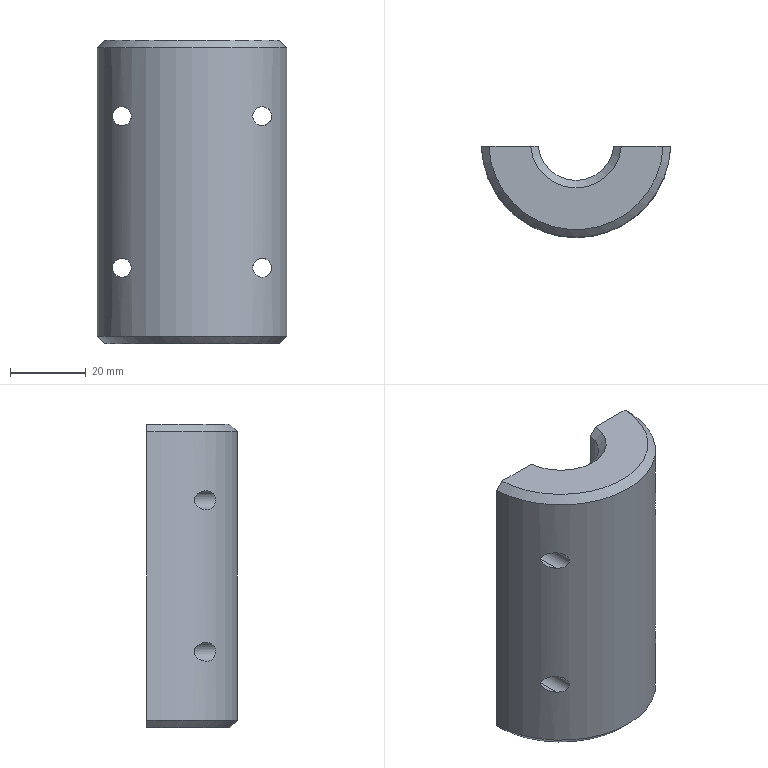Part | SolidWorks | features Chamfer 1, Extrusion 1, HoleWzd 1 | 1 solid | 18 faces | box 49.96 x 24 x 80 mm | volume 61914 mm3 | cylinder 10 | plane 4 | cone 4 | commonest cylinder face diameters 5 x8 20 x1 50 x1
STEP:
#1=CARTESIAN_POINT('',(-18.5,-16.815,17.5));
#2=VERTEX_POINT('',#1);
#3=CARTESIAN_POINT('',(-18.5,-16.815,22.5));
#4=VERTEX_POINT('',#3);
#5=CARTESIAN_POINT('',(-18.5,-16.815,17.5));
#6=CARTESIAN_POINT('',(-18.791,-16.495,17.5));
#7=CARTESIAN_POINT('',(-19.077,-16.163,17.551));
#8=CARTESIAN_POINT('',(-19.612,-15.509,17.743));
#9=CARTESIAN_POINT('',(-19.865,-15.183,17.884));
#10=CARTESIAN_POINT('',(-20.215,-14.711,18.174));
#11=CARTESIAN_POINT('',(-20.325,-14.558,18.284));
#12=CARTESIAN_POINT('',(-20.531,-14.266,18.533));
#13=CARTESIAN_POINT('',(-20.627,-14.126,18.675));
#14=CARTESIAN_POINT('',(-20.794,-13.878,18.991));
#15=CARTESIAN_POINT('',(-20.867,-13.768,19.171));
#16=CARTESIAN_POINT('',(-20.97,-13.611,19.564));
#17=CARTESIAN_POINT('',(-21.,-13.565,19.783));
#18=CARTESIAN_POINT('',(-21.,-13.565,20.109));
#19=CARTESIAN_POINT('',(-20.993,-13.576,20.22));
#20=CARTESIAN_POINT('',(-20.965,-13.619,20.432));
#21=CARTESIAN_POINT('',(-20.944,-13.651,20.535));
#22=CARTESIAN_POINT('',(-20.866,-13.771,20.834));
#23=CARTESIAN_POINT('',(-20.795,-13.878,21.009));
#24=CARTESIAN_POINT('',(-20.625,-14.129,21.329));
#25=CARTESIAN_POINT('',(-20.53,-14.267,21.467));
#26=CARTESIAN_POINT('',(-20.325,-14.557,21.716));
#27=CARTESIAN_POINT('',(-20.214,-14.712,21.826));
#28=CARTESIAN_POINT('',(-19.866,-15.182,22.116));
#29=CARTESIAN_POINT('',(-19.615,-15.505,22.256));
#30=CARTESIAN_POINT('',(-19.213,-15.997,22.4));
#31=CARTESIAN_POINT('',(-19.074,-16.163,22.437));
#32=CARTESIAN_POINT('',(-18.791,-16.491,22.487));
#33=CARTESIAN_POINT('',(-18.647,-16.653,22.5));
#34=CARTESIAN_POINT('',(-18.5,-16.815,22.5));
#35=B_SPLINE_CURVE_WITH_KNOTS('',3,(#5,#6,#7,#8,#9,#10,#11,#12,#13,#14,#15,#16,#17,#18,#19,#20,#21,#22,#23,#24,#25,#26,#27,#28,#29,#30,#31,#32,#33,#34),.UNSPECIFIED.,.F.,.F.,(4,2,2,2,2,2,2,2,2,2,2,2,2,2,4),(0.009381,0.01068,0.01197,0.01262,0.01327,0.01391,0.01456,0.01489,0.01521,0.01586,0.0165,0.01715,0.01845,0.0191,0.01974),.UNSPECIFIED.);
#36=EDGE_CURVE('',#2,#4,#35,.T.);
#37=ORIENTED_EDGE('',*,*,#36,.F.);
#38=CARTESIAN_POINT('',(-18.5,-1.,17.5));
#39=VERTEX_POINT('',#38);
#40=CARTESIAN_POINT('',(-18.5,-1.,17.5));
#41=DIRECTION('',(0.,1.,0.));
#42=VECTOR('',#41,1000.);
#43=LINE('',#40,#42);
#44=EDGE_CURVE('',#2,#39,#43,.T.);
#45=ORIENTED_EDGE('',*,*,#44,.T.);
#46=CARTESIAN_POINT('',(-18.5,-1.,22.5));
#47=VERTEX_POINT('',#46);
#48=CARTESIAN_POINT('',(-18.5,-1.,20.));
#49=DIRECTION('',(0.,1.,0.));
#50=DIRECTION('',(0.,0.,1.));
#51=AXIS2_PLACEMENT_3D('',#48,#49,#50);
#52=CIRCLE('',#51,2.5);
#53=EDGE_CURVE('',#39,#47,#52,.T.);
#54=ORIENTED_EDGE('',*,*,#53,.T.);
#55=CARTESIAN_POINT('',(-18.5,-1.,22.5));
#56=DIRECTION('',(0.,1.,0.));
#57=VECTOR('',#56,1000.);
#58=LINE('',#55,#57);
#59=EDGE_CURVE('',#4,#47,#58,.T.);
#60=ORIENTED_EDGE('',*,*,#59,.F.);
#61=EDGE_LOOP('',(#37,#45,#54,#60));
#62=FACE_OUTER_BOUND('',#61,.T.);
#63=CARTESIAN_POINT('',(-18.5,-1.,20.));
#64=DIRECTION('',(0.,1.,0.));
#65=DIRECTION('',(0.,0.,1.));
#66=AXIS2_PLACEMENT_3D('',#63,#64,#65);
#67=CYLINDRICAL_SURFACE('',#66,2.5);
#68=ADVANCED_FACE('',(#62),#67,.F.);
#69=CARTESIAN_POINT('',(18.5,-16.815,17.5));
#70=VERTEX_POINT('',#69);
#71=CARTESIAN_POINT('',(18.5,-16.815,22.5));
#72=VERTEX_POINT('',#71);
#73=CARTESIAN_POINT('',(18.5,-16.815,17.5));
#74=CARTESIAN_POINT('',(18.235,-17.107,17.5));
#75=CARTESIAN_POINT('',(17.966,-17.388,17.541));
#76=CARTESIAN_POINT('',(17.56,-17.796,17.679));
#77=CARTESIAN_POINT('',(17.424,-17.929,17.738));
#78=CARTESIAN_POINT('',(17.16,-18.181,17.884));
#79=CARTESIAN_POINT('',(17.031,-18.302,17.97));
#80=CARTESIAN_POINT('',(16.783,-18.53,18.176));
#81=CARTESIAN_POINT('',(16.663,-18.637,18.295));
#82=CARTESIAN_POINT('',(16.447,-18.828,18.563));
#83=CARTESIAN_POINT('',(16.348,-18.914,18.714));
#84=CARTESIAN_POINT('',(16.183,-19.056,19.044));
#85=CARTESIAN_POINT('',(16.116,-19.112,19.222));
#86=CARTESIAN_POINT('',(16.024,-19.189,19.602));
#87=CARTESIAN_POINT('',(16.,-19.209,19.796));
#88=CARTESIAN_POINT('',(16.,-19.21,20.193));
#89=CARTESIAN_POINT('',(16.023,-19.19,20.39));
#90=CARTESIAN_POINT('',(16.113,-19.115,20.768));
#91=CARTESIAN_POINT('',(16.18,-19.058,20.949));
#92=CARTESIAN_POINT('',(16.345,-18.917,21.28));
#93=CARTESIAN_POINT('',(16.444,-18.831,21.432));
#94=CARTESIAN_POINT('',(16.66,-18.64,21.702));
#95=CARTESIAN_POINT('',(16.78,-18.533,21.821));
#96=CARTESIAN_POINT('',(17.028,-18.305,22.027));
#97=CARTESIAN_POINT('',(17.157,-18.184,22.114));
#98=CARTESIAN_POINT('',(17.421,-17.932,22.26));
#99=CARTESIAN_POINT('',(17.557,-17.799,22.32));
#100=CARTESIAN_POINT('',(17.964,-17.391,22.458));
#101=CARTESIAN_POINT('',(18.233,-17.109,22.5));
#102=CARTESIAN_POINT('',(18.5,-16.815,22.5));
#103=B_SPLINE_CURVE_WITH_KNOTS('',3,(#73,#74,#75,#76,#77,#78,#79,#80,#81,#82,#83,#84,#85,#86,#87,#88,#89,#90,#91,#92,#93,#94,#95,#96,#97,#98,#99,#100,#101,#102),.UNSPECIFIED.,.F.,.F.,(4,2,2,2,2,2,2,2,2,2,2,2,2,2,4),(0.01037,0.01154,0.01213,0.01271,0.0133,0.01389,0.01447,0.01506,0.01565,0.01623,0.01682,0.01741,0.01799,0.01858,0.01975),.UNSPECIFIED.);
#104=EDGE_CURVE('',#70,#72,#103,.T.);
#105=ORIENTED_EDGE('',*,*,#104,.F.);
#106=CARTESIAN_POINT('',(18.5,-1.,17.5));
#107=VERTEX_POINT('',#106);
#108=CARTESIAN_POINT('',(18.5,-1.,17.5));
#109=DIRECTION('',(0.,1.,0.));
#110=VECTOR('',#109,1000.);
#111=LINE('',#108,#110);
#112=EDGE_CURVE('',#70,#107,#111,.T.);
#113=ORIENTED_EDGE('',*,*,#112,.T.);
#114=CARTESIAN_POINT('',(18.5,-1.,22.5));
#115=VERTEX_POINT('',#114);
#116=CARTESIAN_POINT('',(18.5,-1.,20.));
#117=DIRECTION('',(0.,1.,0.));
#118=DIRECTION('',(0.,0.,1.));
#119=AXIS2_PLACEMENT_3D('',#116,#117,#118);
#120=CIRCLE('',#119,2.5);
#121=EDGE_CURVE('',#107,#115,#120,.T.);
#122=ORIENTED_EDGE('',*,*,#121,.T.);
#123=CARTESIAN_POINT('',(18.5,-1.,22.5));
#124=DIRECTION('',(0.,1.,0.));
#125=VECTOR('',#124,1000.);
#126=LINE('',#123,#125);
#127=EDGE_CURVE('',#72,#115,#126,.T.);
#128=ORIENTED_EDGE('',*,*,#127,.F.);
#129=EDGE_LOOP('',(#105,#113,#122,#128));
#130=FACE_OUTER_BOUND('',#129,.T.);
#131=CARTESIAN_POINT('',(18.5,-1.,20.));
#132=DIRECTION('',(0.,1.,0.));
#133=DIRECTION('',(0.,0.,1.));
#134=AXIS2_PLACEMENT_3D('',#131,#132,#133);
#135=CYLINDRICAL_SURFACE('',#134,2.5);
#136=ADVANCED_FACE('',(#130),#135,.F.);
#137=CARTESIAN_POINT('',(18.5,-16.815,57.5));
#138=VERTEX_POINT('',#137);
#139=CARTESIAN_POINT('',(18.5,-16.815,62.5));
#140=VERTEX_POINT('',#139);
#141=CARTESIAN_POINT('',(18.5,-16.815,57.5));
#142=CARTESIAN_POINT('',(18.235,-17.107,57.5));
#143=CARTESIAN_POINT('',(17.966,-17.388,57.541));
#144=CARTESIAN_POINT('',(17.56,-17.796,57.679));
#145=CARTESIAN_POINT('',(17.424,-17.929,57.738));
#146=CARTESIAN_POINT('',(17.16,-18.181,57.884));
#147=CARTESIAN_POINT('',(17.031,-18.302,57.97));
#148=CARTESIAN_POINT('',(16.783,-18.53,58.176));
#149=CARTESIAN_POINT('',(16.663,-18.637,58.295));
#150=CARTESIAN_POINT('',(16.447,-18.828,58.563));
#151=CARTESIAN_POINT('',(16.348,-18.914,58.714));
#152=CARTESIAN_POINT('',(16.183,-19.056,59.044));
#153=CARTESIAN_POINT('',(16.116,-19.112,59.222));
#154=CARTESIAN_POINT('',(16.024,-19.189,59.602));
#155=CARTESIAN_POINT('',(16.,-19.209,59.796));
#156=CARTESIAN_POINT('',(16.,-19.21,60.193));
#157=CARTESIAN_POINT('',(16.023,-19.19,60.39));
#158=CARTESIAN_POINT('',(16.113,-19.115,60.768));
#159=CARTESIAN_POINT('',(16.18,-19.058,60.949));
#160=CARTESIAN_POINT('',(16.345,-18.917,61.28));
#161=CARTESIAN_POINT('',(16.444,-18.831,61.432));
#162=CARTESIAN_POINT('',(16.66,-18.64,61.702));
#163=CARTESIAN_POINT('',(16.78,-18.533,61.821));
#164=CARTESIAN_POINT('',(17.028,-18.305,62.027));
#165=CARTESIAN_POINT('',(17.157,-18.184,62.114));
#166=CARTESIAN_POINT('',(17.421,-17.932,62.26));
#167=CARTESIAN_POINT('',(17.557,-17.799,62.32));
#168=CARTESIAN_POINT('',(17.964,-17.391,62.458));
#169=CARTESIAN_POINT('',(18.233,-17.109,62.5));
#170=CARTESIAN_POINT('',(18.5,-16.815,62.5));
#171=B_SPLINE_CURVE_WITH_KNOTS('',3,(#141,#142,#143,#144,#145,#146,#147,#148,#149,#150,#151,#152,#153,#154,#155,#156,#157,#158,#159,#160,#161,#162,#163,#164,#165,#166,#167,#168,#169,#170),.UNSPECIFIED.,.F.,.F.,(4,2,2,2,2,2,2,2,2,2,2,2,2,2,4),(0.01037,0.01154,0.01213,0.01271,0.0133,0.01389,0.01447,0.01506,0.01565,0.01623,0.01682,0.01741,0.01799,0.01858,0.01975),.UNSPECIFIED.);
#172=EDGE_CURVE('',#138,#140,#171,.T.);
#173=ORIENTED_EDGE('',*,*,#172,.F.);
#174=CARTESIAN_POINT('',(18.5,-1.,57.5));
#175=VERTEX_POINT('',#174);
#176=CARTESIAN_POINT('',(18.5,-1.,57.5));
#177=DIRECTION('',(0.,1.,0.));
#178=VECTOR('',#177,1000.);
#179=LINE('',#176,#178);
#180=EDGE_CURVE('',#138,#175,#179,.T.);
#181=ORIENTED_EDGE('',*,*,#180,.T.);
#182=CARTESIAN_POINT('',(18.5,-1.,62.5));
#183=VERTEX_POINT('',#182);
#184=CARTESIAN_POINT('',(18.5,-1.,60.));
#185=DIRECTION('',(0.,1.,0.));
#186=DIRECTION('',(0.,0.,1.));
#187=AXIS2_PLACEMENT_3D('',#184,#185,#186);
#188=CIRCLE('',#187,2.5);
#189=EDGE_CURVE('',#175,#183,#188,.T.);
#190=ORIENTED_EDGE('',*,*,#189,.T.);
#191=CARTESIAN_POINT('',(18.5,-1.,62.5));
#192=DIRECTION('',(0.,1.,0.));
#193=VECTOR('',#192,1000.);
#194=LINE('',#191,#193);
#195=EDGE_CURVE('',#140,#183,#194,.T.);
#196=ORIENTED_EDGE('',*,*,#195,.F.);
#197=EDGE_LOOP('',(#173,#181,#190,#196));
#198=FACE_OUTER_BOUND('',#197,.T.);
#199=CARTESIAN_POINT('',(18.5,-1.,60.));
#200=DIRECTION('',(0.,1.,0.));
#201=DIRECTION('',(0.,0.,1.));
#202=AXIS2_PLACEMENT_3D('',#199,#200,#201);
#203=CYLINDRICAL_SURFACE('',#202,2.5);
#204=ADVANCED_FACE('',(#198),#203,.F.);
#205=CARTESIAN_POINT('',(-18.5,-16.815,57.5));
#206=VERTEX_POINT('',#205);
#207=CARTESIAN_POINT('',(-18.5,-16.815,62.5));
#208=VERTEX_POINT('',#207);
#209=CARTESIAN_POINT('',(-18.5,-16.815,57.5));
#210=CARTESIAN_POINT('',(-18.791,-16.495,57.5));
#211=CARTESIAN_POINT('',(-19.077,-16.163,57.551));
#212=CARTESIAN_POINT('',(-19.612,-15.509,57.743));
#213=CARTESIAN_POINT('',(-19.865,-15.183,57.884));
#214=CARTESIAN_POINT('',(-20.215,-14.711,58.174));
#215=CARTESIAN_POINT('',(-20.325,-14.558,58.284));
#216=CARTESIAN_POINT('',(-20.531,-14.266,58.533));
#217=CARTESIAN_POINT('',(-20.627,-14.126,58.675));
#218=CARTESIAN_POINT('',(-20.794,-13.878,58.991));
#219=CARTESIAN_POINT('',(-20.867,-13.768,59.171));
#220=CARTESIAN_POINT('',(-20.97,-13.611,59.564));
#221=CARTESIAN_POINT('',(-21.,-13.565,59.783));
#222=CARTESIAN_POINT('',(-21.,-13.565,60.109));
#223=CARTESIAN_POINT('',(-20.993,-13.576,60.22));
#224=CARTESIAN_POINT('',(-20.965,-13.619,60.432));
#225=CARTESIAN_POINT('',(-20.944,-13.651,60.535));
#226=CARTESIAN_POINT('',(-20.866,-13.771,60.834));
#227=CARTESIAN_POINT('',(-20.795,-13.878,61.009));
#228=CARTESIAN_POINT('',(-20.625,-14.129,61.329));
#229=CARTESIAN_POINT('',(-20.53,-14.267,61.467));
#230=CARTESIAN_POINT('',(-20.325,-14.557,61.716));
#231=CARTESIAN_POINT('',(-20.214,-14.712,61.826));
#232=CARTESIAN_POINT('',(-19.866,-15.182,62.116));
#233=CARTESIAN_POINT('',(-19.615,-15.505,62.256));
#234=CARTESIAN_POINT('',(-19.213,-15.997,62.4));
#235=CARTESIAN_POINT('',(-19.074,-16.163,62.437));
#236=CARTESIAN_POINT('',(-18.791,-16.491,62.487));
#237=CARTESIAN_POINT('',(-18.647,-16.653,62.5));
#238=CARTESIAN_POINT('',(-18.5,-16.815,62.5));
#239=B_SPLINE_CURVE_WITH_KNOTS('',3,(#209,#210,#211,#212,#213,#214,#215,#216,#217,#218,#219,#220,#221,#222,#223,#224,#225,#226,#227,#228,#229,#230,#231,#232,#233,#234,#235,#236,#237,#238),.UNSPECIFIED.,.F.,.F.,(4,2,2,2,2,2,2,2,2,2,2,2,2,2,4),(0.009381,0.01068,0.01197,0.01262,0.01327,0.01391,0.01456,0.01489,0.01521,0.01586,0.0165,0.01715,0.01845,0.0191,0.01974),.UNSPECIFIED.);
#240=EDGE_CURVE('',#206,#208,#239,.T.);
#241=ORIENTED_EDGE('',*,*,#240,.F.);
#242=CARTESIAN_POINT('',(-18.5,-1.,57.5));
#243=VERTEX_POINT('',#242);
#244=CARTESIAN_POINT('',(-18.5,-1.,57.5));
#245=DIRECTION('',(0.,1.,0.));
#246=VECTOR('',#245,1000.);
#247=LINE('',#244,#246);
#248=EDGE_CURVE('',#206,#243,#247,.T.);
#249=ORIENTED_EDGE('',*,*,#248,.T.);
#250=CARTESIAN_POINT('',(-18.5,-1.,62.5));
#251=VERTEX_POINT('',#250);
#252=CARTESIAN_POINT('',(-18.5,-1.,60.));
#253=DIRECTION('',(0.,1.,0.));
#254=DIRECTION('',(0.,0.,1.));
#255=AXIS2_PLACEMENT_3D('',#252,#253,#254);
#256=CIRCLE('',#255,2.5);
#257=EDGE_CURVE('',#243,#251,#256,.T.);
#258=ORIENTED_EDGE('',*,*,#257,.T.);
#259=CARTESIAN_POINT('',(-18.5,-1.,62.5));
#260=DIRECTION('',(0.,1.,0.));
#261=VECTOR('',#260,1000.);
#262=LINE('',#259,#261);
#263=EDGE_CURVE('',#208,#251,#262,.T.);
#264=ORIENTED_EDGE('',*,*,#263,.F.);
#265=EDGE_LOOP('',(#241,#249,#258,#264));
#266=FACE_OUTER_BOUND('',#265,.T.);
#267=CARTESIAN_POINT('',(-18.5,-1.,60.));
#268=DIRECTION('',(0.,1.,0.));
#269=DIRECTION('',(0.,0.,1.));
#270=AXIS2_PLACEMENT_3D('',#267,#268,#269);
#271=CYLINDRICAL_SURFACE('',#270,2.5);
#272=ADVANCED_FACE('',(#266),#271,.F.);
#273=CARTESIAN_POINT('',(-9.95,-1.,78.));
#274=VERTEX_POINT('',#273);
#275=CARTESIAN_POINT('',(-9.95,-1.,2.));
#276=VERTEX_POINT('',#275);
#277=CARTESIAN_POINT('',(-9.95,-1.,80.));
#278=DIRECTION('',(0.,0.,-1.));
#279=VECTOR('',#278,1000.);
#280=LINE('',#277,#279);
#281=EDGE_CURVE('',#274,#276,#280,.T.);
#282=ORIENTED_EDGE('',*,*,#281,.F.);
#283=CARTESIAN_POINT('',(9.95,-1.,78.));
#284=VERTEX_POINT('',#283);
#285=CARTESIAN_POINT('',(0.,0.,78.));
#286=DIRECTION('',(0.,0.,1.));
#287=DIRECTION('',(1.,0.,0.));
#288=AXIS2_PLACEMENT_3D('',#285,#286,#287);
#289=CIRCLE('',#288,10.);
#290=EDGE_CURVE('',#274,#284,#289,.T.);
#291=ORIENTED_EDGE('',*,*,#290,.T.);
#292=CARTESIAN_POINT('',(9.95,-1.,2.));
#293=VERTEX_POINT('',#292);
#294=CARTESIAN_POINT('',(9.95,-1.,80.));
#295=DIRECTION('',(0.,0.,-1.));
#296=VECTOR('',#295,1000.);
#297=LINE('',#294,#296);
#298=EDGE_CURVE('',#284,#293,#297,.T.);
#299=ORIENTED_EDGE('',*,*,#298,.T.);
#300=CARTESIAN_POINT('',(0.,0.,2.));
#301=DIRECTION('',(0.,0.,-1.));
#302=DIRECTION('',(1.,0.,0.));
#303=AXIS2_PLACEMENT_3D('',#300,#301,#302);
#304=CIRCLE('',#303,10.);
#305=EDGE_CURVE('',#293,#276,#304,.T.);
#306=ORIENTED_EDGE('',*,*,#305,.T.);
#307=EDGE_LOOP('',(#282,#291,#299,#306));
#308=FACE_OUTER_BOUND('',#307,.T.);
#309=CARTESIAN_POINT('',(0.,0.,80.));
#310=DIRECTION('',(0.,0.,-1.));
#311=DIRECTION('',(-1.,0.,0.));
#312=AXIS2_PLACEMENT_3D('',#309,#310,#311);
#313=CYLINDRICAL_SURFACE('',#312,10.);
#314=ADVANCED_FACE('',(#308),#313,.F.);
#315=CARTESIAN_POINT('',(-18.5,-1.,20.));
#316=DIRECTION('',(0.,1.,0.));
#317=DIRECTION('',(0.,0.,1.));
#318=AXIS2_PLACEMENT_3D('',#315,#316,#317);
#319=CIRCLE('',#318,2.5);
#320=EDGE_CURVE('',#47,#39,#319,.T.);
#321=ORIENTED_EDGE('',*,*,#320,.F.);
#322=ORIENTED_EDGE('',*,*,#53,.F.);
#323=EDGE_LOOP('',(#321,#322));
#324=FACE_BOUND('',#323,.T.);
#325=CARTESIAN_POINT('',(-18.5,-1.,60.));
#326=DIRECTION('',(0.,1.,0.));
#327=DIRECTION('',(0.,0.,1.));
#328=AXIS2_PLACEMENT_3D('',#325,#326,#327);
#329=CIRCLE('',#328,2.5);
#330=EDGE_CURVE('',#251,#243,#329,.T.);
#331=ORIENTED_EDGE('',*,*,#330,.F.);
#332=ORIENTED_EDGE('',*,*,#257,.F.);
#333=EDGE_LOOP('',(#331,#332));
#334=FACE_BOUND('',#333,.T.);
#335=CARTESIAN_POINT('',(-24.98,-1.,78.));
#336=VERTEX_POINT('',#335);
#337=CARTESIAN_POINT('',(-24.98,-1.,2.));
#338=VERTEX_POINT('',#337);
#339=CARTESIAN_POINT('',(-24.98,-1.,80.));
#340=DIRECTION('',(0.,0.,-1.));
#341=VECTOR('',#340,1000.);
#342=LINE('',#339,#341);
#343=EDGE_CURVE('',#336,#338,#342,.T.);
#344=ORIENTED_EDGE('',*,*,#343,.F.);
#345=CARTESIAN_POINT('',(-22.978,-1.,80.));
#346=VERTEX_POINT('',#345);
#347=CARTESIAN_POINT('',(-24.98,-1.,78.));
#348=CARTESIAN_POINT('',(-24.313,-1.,78.667));
#349=CARTESIAN_POINT('',(-23.646,-1.,79.333));
#350=CARTESIAN_POINT('',(-22.978,-1.,80.));
#351=B_SPLINE_CURVE_WITH_KNOTS('',3,(#347,#348,#349,#350),.UNSPECIFIED.,.F.,.F.,(4,4),(0.,0.00283),.UNSPECIFIED.);
#352=EDGE_CURVE('',#336,#346,#351,.T.);
#353=ORIENTED_EDGE('',*,*,#352,.T.);
#354=CARTESIAN_POINT('',(-11.958,-1.,80.));
#355=VERTEX_POINT('',#354);
#356=CARTESIAN_POINT('',(-24.98,-1.,80.));
#357=DIRECTION('',(-1.,0.,0.));
#358=VECTOR('',#357,1000.);
#359=LINE('',#356,#358);
#360=EDGE_CURVE('',#355,#346,#359,.T.);
#361=ORIENTED_EDGE('',*,*,#360,.F.);
#362=CARTESIAN_POINT('',(-11.958,-1.,80.));
#363=CARTESIAN_POINT('',(-11.289,-1.,79.333));
#364=CARTESIAN_POINT('',(-10.62,-1.,78.666));
#365=CARTESIAN_POINT('',(-9.95,-1.,78.));
#366=B_SPLINE_CURVE_WITH_KNOTS('',3,(#362,#363,#364,#365),.UNSPECIFIED.,.F.,.F.,(4,4),(0.,0.002834),.UNSPECIFIED.);
#367=EDGE_CURVE('',#355,#274,#366,.T.);
#368=ORIENTED_EDGE('',*,*,#367,.T.);
#369=ORIENTED_EDGE('',*,*,#281,.T.);
#370=CARTESIAN_POINT('',(-11.958,-1.,0.));
#371=VERTEX_POINT('',#370);
#372=CARTESIAN_POINT('',(-9.95,-1.,2.));
#373=CARTESIAN_POINT('',(-10.62,-1.,1.334));
#374=CARTESIAN_POINT('',(-11.289,-1.,0.6669));
#375=CARTESIAN_POINT('',(-11.958,-1.,0.));
#376=B_SPLINE_CURVE_WITH_KNOTS('',3,(#372,#373,#374,#375),.UNSPECIFIED.,.F.,.F.,(4,4),(0.,0.002834),.UNSPECIFIED.);
#377=EDGE_CURVE('',#276,#371,#376,.T.);
#378=ORIENTED_EDGE('',*,*,#377,.T.);
#379=CARTESIAN_POINT('',(-22.978,-1.,0.));
#380=VERTEX_POINT('',#379);
#381=CARTESIAN_POINT('',(-24.98,-1.,0.));
#382=DIRECTION('',(-1.,0.,0.));
#383=VECTOR('',#382,1000.);
#384=LINE('',#381,#383);
#385=EDGE_CURVE('',#371,#380,#384,.T.);
#386=ORIENTED_EDGE('',*,*,#385,.T.);
#387=CARTESIAN_POINT('',(-22.978,-1.,0.));
#388=CARTESIAN_POINT('',(-23.646,-1.,0.6666));
#389=CARTESIAN_POINT('',(-24.313,-1.,1.333));
#390=CARTESIAN_POINT('',(-24.98,-1.,2.));
#391=B_SPLINE_CURVE_WITH_KNOTS('',3,(#387,#388,#389,#390),.UNSPECIFIED.,.F.,.F.,(4,4),(0.,0.00283),.UNSPECIFIED.);
#392=EDGE_CURVE('',#380,#338,#391,.T.);
#393=ORIENTED_EDGE('',*,*,#392,.T.);
#394=EDGE_LOOP('',(#344,#353,#361,#368,#369,#378,#386,#393));
#395=FACE_OUTER_BOUND('',#394,.T.);
#396=CARTESIAN_POINT('',(-24.98,-1.,80.));
#397=DIRECTION('',(0.,-1.,0.));
#398=DIRECTION('',(0.,0.,-1.));
#399=AXIS2_PLACEMENT_3D('',#396,#397,#398);
#400=PLANE('',#399);
#401=ADVANCED_FACE('',(#324,#334,#395),#400,.F.);
#402=CARTESIAN_POINT('',(-18.5,-16.815,22.5));
#403=CARTESIAN_POINT('',(-18.233,-17.108,22.5));
#404=CARTESIAN_POINT('',(-17.965,-17.39,22.459));
#405=CARTESIAN_POINT('',(-17.561,-17.795,22.321));
#406=CARTESIAN_POINT('',(-17.425,-17.928,22.262));
#407=CARTESIAN_POINT('',(-17.16,-18.182,22.116));
#408=CARTESIAN_POINT('',(-17.031,-18.303,22.029));
#409=CARTESIAN_POINT('',(-16.783,-18.53,21.824));
#410=CARTESIAN_POINT('',(-16.663,-18.638,21.704));
#411=CARTESIAN_POINT('',(-16.446,-18.829,21.436));
#412=CARTESIAN_POINT('',(-16.348,-18.914,21.287));
#413=CARTESIAN_POINT('',(-16.181,-19.057,20.953));
#414=CARTESIAN_POINT('',(-16.116,-19.113,20.776));
#415=CARTESIAN_POINT('',(-16.024,-19.189,20.397));
#416=CARTESIAN_POINT('',(-16.,-19.209,20.2));
#417=CARTESIAN_POINT('',(-16.,-19.21,19.805));
#418=CARTESIAN_POINT('',(-16.024,-19.19,19.606));
#419=CARTESIAN_POINT('',(-16.114,-19.114,19.229));
#420=CARTESIAN_POINT('',(-16.181,-19.057,19.047));
#421=CARTESIAN_POINT('',(-16.347,-18.916,18.717));
#422=CARTESIAN_POINT('',(-16.446,-18.829,18.564));
#423=CARTESIAN_POINT('',(-16.663,-18.638,18.296));
#424=CARTESIAN_POINT('',(-16.78,-18.532,18.178));
#425=CARTESIAN_POINT('',(-17.03,-18.304,17.972));
#426=CARTESIAN_POINT('',(-17.16,-18.182,17.884));
#427=CARTESIAN_POINT('',(-17.423,-17.929,17.739));
#428=CARTESIAN_POINT('',(-17.557,-17.798,17.68));
#429=CARTESIAN_POINT('',(-17.829,-17.526,17.588));
#430=CARTESIAN_POINT('',(-17.966,-17.386,17.554));
#431=CARTESIAN_POINT('',(-18.235,-17.103,17.51));
#432=CARTESIAN_POINT('',(-18.368,-16.96,17.5));
#433=CARTESIAN_POINT('',(-18.5,-16.815,17.5));
#434=B_SPLINE_CURVE_WITH_KNOTS('',3,(#402,#403,#404,#405,#406,#407,#408,#409,#410,#411,#412,#413,#414,#415,#416,#417,#418,#419,#420,#421,#422,#423,#424,#425,#426,#427,#428,#429,#430,#431,#432,#433),.UNSPECIFIED.,.F.,.F.,(4,2,2,2,2,2,2,2,2,2,2,2,2,2,2,4),(0.,0.001173,0.001759,0.002345,0.002931,0.003518,0.004104,0.00469,0.005277,0.005863,0.006449,0.007035,0.007622,0.008208,0.008794,0.009381),.UNSPECIFIED.);
#435=EDGE_CURVE('',#4,#2,#434,.T.);
#436=ORIENTED_EDGE('',*,*,#435,.T.);
#437=ORIENTED_EDGE('',*,*,#36,.T.);
#438=EDGE_LOOP('',(#436,#437));
#439=FACE_BOUND('',#438,.T.);
#440=CARTESIAN_POINT('',(18.5,-16.815,22.5));
#441=CARTESIAN_POINT('',(18.795,-16.491,22.5));
#442=CARTESIAN_POINT('',(19.075,-16.165,22.449));
#443=CARTESIAN_POINT('',(19.61,-15.512,22.258));
#444=CARTESIAN_POINT('',(19.866,-15.182,22.115));
#445=CARTESIAN_POINT('',(20.213,-14.713,21.827));
#446=CARTESIAN_POINT('',(20.323,-14.56,21.718));
#447=CARTESIAN_POINT('',(20.531,-14.266,21.467));
#448=CARTESIAN_POINT('',(20.626,-14.128,21.327));
#449=CARTESIAN_POINT('',(20.794,-13.879,21.01));
#450=CARTESIAN_POINT('',(20.867,-13.769,20.831));
#451=CARTESIAN_POINT('',(20.97,-13.611,20.436));
#452=CARTESIAN_POINT('',(21.,-13.564,20.219));
#453=CARTESIAN_POINT('',(21.,-13.565,19.888));
#454=CARTESIAN_POINT('',(20.993,-13.576,19.78));
#455=CARTESIAN_POINT('',(20.965,-13.619,19.567));
#456=CARTESIAN_POINT('',(20.944,-13.651,19.463));
#457=CARTESIAN_POINT('',(20.866,-13.77,19.168));
#458=CARTESIAN_POINT('',(20.793,-13.88,18.989));
#459=CARTESIAN_POINT('',(20.626,-14.128,18.672));
#460=CARTESIAN_POINT('',(20.531,-14.266,18.533));
#461=CARTESIAN_POINT('',(20.324,-14.56,18.282));
#462=CARTESIAN_POINT('',(20.214,-14.712,18.174));
#463=CARTESIAN_POINT('',(19.868,-15.18,17.886));
#464=CARTESIAN_POINT('',(19.612,-15.509,17.743));
#465=CARTESIAN_POINT('',(19.21,-16.,17.599));
#466=CARTESIAN_POINT('',(19.073,-16.164,17.562));
#467=CARTESIAN_POINT('',(18.791,-16.49,17.513));
#468=CARTESIAN_POINT('',(18.646,-16.654,17.5));
#469=CARTESIAN_POINT('',(18.5,-16.815,17.5));
#470=B_SPLINE_CURVE_WITH_KNOTS('',3,(#440,#441,#442,#443,#444,#445,#446,#447,#448,#449,#450,#451,#452,#453,#454,#455,#456,#457,#458,#459,#460,#461,#462,#463,#464,#465,#466,#467,#468,#469),.UNSPECIFIED.,.F.,.F.,(4,2,2,2,2,2,2,2,2,2,2,2,2,2,4),(0.,0.001296,0.002592,0.00324,0.003888,0.004535,0.005183,0.005507,0.005831,0.006479,0.007127,0.007775,0.009071,0.009719,0.01037),.UNSPECIFIED.);
#471=EDGE_CURVE('',#72,#70,#470,.T.);
#472=ORIENTED_EDGE('',*,*,#471,.T.);
#473=ORIENTED_EDGE('',*,*,#104,.T.);
#474=EDGE_LOOP('',(#472,#473));
#475=FACE_BOUND('',#474,.T.);
#476=CARTESIAN_POINT('',(18.5,-16.815,62.5));
#477=CARTESIAN_POINT('',(18.795,-16.491,62.5));
#478=CARTESIAN_POINT('',(19.075,-16.165,62.449));
#479=CARTESIAN_POINT('',(19.61,-15.512,62.258));
#480=CARTESIAN_POINT('',(19.866,-15.182,62.115));
#481=CARTESIAN_POINT('',(20.213,-14.713,61.827));
#482=CARTESIAN_POINT('',(20.323,-14.56,61.718));
#483=CARTESIAN_POINT('',(20.531,-14.266,61.467));
#484=CARTESIAN_POINT('',(20.626,-14.128,61.327));
#485=CARTESIAN_POINT('',(20.794,-13.879,61.01));
#486=CARTESIAN_POINT('',(20.867,-13.769,60.831));
#487=CARTESIAN_POINT('',(20.97,-13.611,60.436));
#488=CARTESIAN_POINT('',(21.,-13.564,60.219));
#489=CARTESIAN_POINT('',(21.,-13.565,59.888));
#490=CARTESIAN_POINT('',(20.993,-13.576,59.78));
#491=CARTESIAN_POINT('',(20.965,-13.619,59.567));
#492=CARTESIAN_POINT('',(20.944,-13.651,59.463));
#493=CARTESIAN_POINT('',(20.866,-13.77,59.168));
#494=CARTESIAN_POINT('',(20.793,-13.88,58.989));
#495=CARTESIAN_POINT('',(20.626,-14.128,58.672));
#496=CARTESIAN_POINT('',(20.531,-14.266,58.533));
#497=CARTESIAN_POINT('',(20.324,-14.56,58.282));
#498=CARTESIAN_POINT('',(20.214,-14.712,58.174));
#499=CARTESIAN_POINT('',(19.868,-15.18,57.886));
#500=CARTESIAN_POINT('',(19.612,-15.509,57.743));
#501=CARTESIAN_POINT('',(19.21,-16.,57.599));
#502=CARTESIAN_POINT('',(19.073,-16.164,57.562));
#503=CARTESIAN_POINT('',(18.791,-16.49,57.513));
#504=CARTESIAN_POINT('',(18.646,-16.654,57.5));
#505=CARTESIAN_POINT('',(18.5,-16.815,57.5));
#506=B_SPLINE_CURVE_WITH_KNOTS('',3,(#476,#477,#478,#479,#480,#481,#482,#483,#484,#485,#486,#487,#488,#489,#490,#491,#492,#493,#494,#495,#496,#497,#498,#499,#500,#501,#502,#503,#504,#505),.UNSPECIFIED.,.F.,.F.,(4,2,2,2,2,2,2,2,2,2,2,2,2,2,4),(0.,0.001296,0.002592,0.00324,0.003888,0.004535,0.005183,0.005507,0.005831,0.006479,0.007127,0.007775,0.009071,0.009719,0.01037),.UNSPECIFIED.);
#507=EDGE_CURVE('',#140,#138,#506,.T.);
#508=ORIENTED_EDGE('',*,*,#507,.T.);
#509=ORIENTED_EDGE('',*,*,#172,.T.);
#510=EDGE_LOOP('',(#508,#509));
#511=FACE_BOUND('',#510,.T.);
#512=CARTESIAN_POINT('',(-18.5,-16.815,62.5));
#513=CARTESIAN_POINT('',(-18.233,-17.108,62.5));
#514=CARTESIAN_POINT('',(-17.965,-17.39,62.459));
#515=CARTESIAN_POINT('',(-17.561,-17.795,62.321));
#516=CARTESIAN_POINT('',(-17.425,-17.928,62.262));
#517=CARTESIAN_POINT('',(-17.16,-18.182,62.116));
#518=CARTESIAN_POINT('',(-17.031,-18.303,62.029));
#519=CARTESIAN_POINT('',(-16.783,-18.53,61.824));
#520=CARTESIAN_POINT('',(-16.663,-18.638,61.704));
#521=CARTESIAN_POINT('',(-16.446,-18.829,61.436));
#522=CARTESIAN_POINT('',(-16.348,-18.914,61.287));
#523=CARTESIAN_POINT('',(-16.181,-19.057,60.953));
#524=CARTESIAN_POINT('',(-16.116,-19.113,60.776));
#525=CARTESIAN_POINT('',(-16.024,-19.189,60.397));
#526=CARTESIAN_POINT('',(-16.,-19.209,60.2));
#527=CARTESIAN_POINT('',(-16.,-19.21,59.805));
#528=CARTESIAN_POINT('',(-16.024,-19.19,59.606));
#529=CARTESIAN_POINT('',(-16.114,-19.114,59.229));
#530=CARTESIAN_POINT('',(-16.181,-19.057,59.047));
#531=CARTESIAN_POINT('',(-16.347,-18.916,58.717));
#532=CARTESIAN_POINT('',(-16.446,-18.829,58.564));
#533=CARTESIAN_POINT('',(-16.663,-18.638,58.296));
#534=CARTESIAN_POINT('',(-16.78,-18.532,58.178));
#535=CARTESIAN_POINT('',(-17.03,-18.304,57.972));
#536=CARTESIAN_POINT('',(-17.16,-18.182,57.884));
#537=CARTESIAN_POINT('',(-17.423,-17.929,57.739));
#538=CARTESIAN_POINT('',(-17.557,-17.798,57.68));
#539=CARTESIAN_POINT('',(-17.829,-17.526,57.588));
#540=CARTESIAN_POINT('',(-17.966,-17.386,57.554));
#541=CARTESIAN_POINT('',(-18.235,-17.103,57.51));
#542=CARTESIAN_POINT('',(-18.368,-16.96,57.5));
#543=CARTESIAN_POINT('',(-18.5,-16.815,57.5));
#544=B_SPLINE_CURVE_WITH_KNOTS('',3,(#512,#513,#514,#515,#516,#517,#518,#519,#520,#521,#522,#523,#524,#525,#526,#527,#528,#529,#530,#531,#532,#533,#534,#535,#536,#537,#538,#539,#540,#541,#542,#543),.UNSPECIFIED.,.F.,.F.,(4,2,2,2,2,2,2,2,2,2,2,2,2,2,2,4),(0.,0.001173,0.001759,0.002345,0.002931,0.003518,0.004104,0.00469,0.005277,0.005863,0.006449,0.007035,0.007622,0.008208,0.008794,0.009381),.UNSPECIFIED.);
#545=EDGE_CURVE('',#208,#206,#544,.T.);
#546=ORIENTED_EDGE('',*,*,#545,.T.);
#547=ORIENTED_EDGE('',*,*,#240,.T.);
#548=EDGE_LOOP('',(#546,#547));
#549=FACE_BOUND('',#548,.T.);
#550=CARTESIAN_POINT('',(24.98,-1.,78.));
#551=VERTEX_POINT('',#550);
#552=CARTESIAN_POINT('',(24.98,-1.,2.));
#553=VERTEX_POINT('',#552);
#554=CARTESIAN_POINT('',(24.98,-1.,80.));
#555=DIRECTION('',(0.,0.,-1.));
#556=VECTOR('',#555,1000.);
#557=LINE('',#554,#556);
#558=EDGE_CURVE('',#551,#553,#557,.T.);
#559=ORIENTED_EDGE('',*,*,#558,.F.);
#560=CARTESIAN_POINT('',(0.,0.,78.));
#561=DIRECTION('',(0.,0.,-1.));
#562=DIRECTION('',(1.,0.,0.));
#563=AXIS2_PLACEMENT_3D('',#560,#561,#562);
#564=CIRCLE('',#563,25.);
#565=EDGE_CURVE('',#551,#336,#564,.T.);
#566=ORIENTED_EDGE('',*,*,#565,.T.);
#567=ORIENTED_EDGE('',*,*,#343,.T.);
#568=CARTESIAN_POINT('',(0.,0.,2.));
#569=DIRECTION('',(0.,0.,1.));
#570=DIRECTION('',(1.,0.,0.));
#571=AXIS2_PLACEMENT_3D('',#568,#569,#570);
#572=CIRCLE('',#571,25.);
#573=EDGE_CURVE('',#338,#553,#572,.T.);
#574=ORIENTED_EDGE('',*,*,#573,.T.);
#575=EDGE_LOOP('',(#559,#566,#567,#574));
#576=FACE_OUTER_BOUND('',#575,.T.);
#577=CARTESIAN_POINT('',(0.,0.,80.));
#578=DIRECTION('',(0.,0.,-1.));
#579=DIRECTION('',(-1.,0.,0.));
#580=AXIS2_PLACEMENT_3D('',#577,#578,#579);
#581=CYLINDRICAL_SURFACE('',#580,25.);
#582=ADVANCED_FACE('',(#439,#475,#511,#549,#576),#581,.T.);
#583=CARTESIAN_POINT('',(18.5,-1.,20.));
#584=DIRECTION('',(0.,1.,0.));
#585=DIRECTION('',(0.,0.,1.));
#586=AXIS2_PLACEMENT_3D('',#583,#584,#585);
#587=CIRCLE('',#586,2.5);
#588=EDGE_CURVE('',#115,#107,#587,.T.);
#589=ORIENTED_EDGE('',*,*,#588,.F.);
#590=ORIENTED_EDGE('',*,*,#121,.F.);
#591=EDGE_LOOP('',(#589,#590));
#592=FACE_BOUND('',#591,.T.);
#593=CARTESIAN_POINT('',(18.5,-1.,60.));
#594=DIRECTION('',(0.,1.,0.));
#595=DIRECTION('',(0.,0.,1.));
#596=AXIS2_PLACEMENT_3D('',#593,#594,#595);
#597=CIRCLE('',#596,2.5);
#598=EDGE_CURVE('',#183,#175,#597,.T.);
#599=ORIENTED_EDGE('',*,*,#598,.F.);
#600=ORIENTED_EDGE('',*,*,#189,.F.);
#601=EDGE_LOOP('',(#599,#600));
#602=FACE_BOUND('',#601,.T.);
#603=CARTESIAN_POINT('',(22.978,-1.,80.));
#604=VERTEX_POINT('',#603);
#605=CARTESIAN_POINT('',(11.958,-1.,80.));
#606=VERTEX_POINT('',#605);
#607=CARTESIAN_POINT('',(9.95,-1.,80.));
#608=DIRECTION('',(-1.,0.,0.));
#609=VECTOR('',#608,1000.);
#610=LINE('',#607,#609);
#611=EDGE_CURVE('',#604,#606,#610,.T.);
#612=ORIENTED_EDGE('',*,*,#611,.F.);
#613=CARTESIAN_POINT('',(22.978,-1.,80.));
#614=CARTESIAN_POINT('',(23.646,-1.,79.333));
#615=CARTESIAN_POINT('',(24.313,-1.,78.667));
#616=CARTESIAN_POINT('',(24.98,-1.,78.));
#617=B_SPLINE_CURVE_WITH_KNOTS('',3,(#613,#614,#615,#616),.UNSPECIFIED.,.F.,.F.,(4,4),(0.,0.00283),.UNSPECIFIED.);
#618=EDGE_CURVE('',#604,#551,#617,.T.);
#619=ORIENTED_EDGE('',*,*,#618,.T.);
#620=ORIENTED_EDGE('',*,*,#558,.T.);
#621=CARTESIAN_POINT('',(22.978,-1.,0.));
#622=VERTEX_POINT('',#621);
#623=CARTESIAN_POINT('',(24.98,-1.,2.));
#624=CARTESIAN_POINT('',(24.313,-1.,1.333));
#625=CARTESIAN_POINT('',(23.646,-1.,0.6666));
#626=CARTESIAN_POINT('',(22.978,-1.,0.));
#627=B_SPLINE_CURVE_WITH_KNOTS('',3,(#623,#624,#625,#626),.UNSPECIFIED.,.F.,.F.,(4,4),(0.,0.00283),.UNSPECIFIED.);
#628=EDGE_CURVE('',#553,#622,#627,.T.);
#629=ORIENTED_EDGE('',*,*,#628,.T.);
#630=CARTESIAN_POINT('',(11.958,-1.,0.));
#631=VERTEX_POINT('',#630);
#632=CARTESIAN_POINT('',(9.95,-1.,0.));
#633=DIRECTION('',(-1.,0.,0.));
#634=VECTOR('',#633,1000.);
#635=LINE('',#632,#634);
#636=EDGE_CURVE('',#622,#631,#635,.T.);
#637=ORIENTED_EDGE('',*,*,#636,.T.);
#638=CARTESIAN_POINT('',(11.958,-1.,0.));
#639=CARTESIAN_POINT('',(11.289,-1.,0.6669));
#640=CARTESIAN_POINT('',(10.62,-1.,1.334));
#641=CARTESIAN_POINT('',(9.95,-1.,2.));
#642=B_SPLINE_CURVE_WITH_KNOTS('',3,(#638,#639,#640,#641),.UNSPECIFIED.,.F.,.F.,(4,4),(0.,0.002834),.UNSPECIFIED.);
#643=EDGE_CURVE('',#631,#293,#642,.T.);
#644=ORIENTED_EDGE('',*,*,#643,.T.);
#645=ORIENTED_EDGE('',*,*,#298,.F.);
#646=CARTESIAN_POINT('',(9.95,-1.,78.));
#647=CARTESIAN_POINT('',(10.62,-1.,78.666));
#648=CARTESIAN_POINT('',(11.289,-1.,79.333));
#649=CARTESIAN_POINT('',(11.958,-1.,80.));
#650=B_SPLINE_CURVE_WITH_KNOTS('',3,(#646,#647,#648,#649),.UNSPECIFIED.,.F.,.F.,(4,4),(0.,0.002834),.UNSPECIFIED.);
#651=EDGE_CURVE('',#284,#606,#650,.T.);
#652=ORIENTED_EDGE('',*,*,#651,.T.);
#653=EDGE_LOOP('',(#612,#619,#620,#629,#637,#644,#645,#652));
#654=FACE_OUTER_BOUND('',#653,.T.);
#655=CARTESIAN_POINT('',(9.95,-1.,80.));
#656=DIRECTION('',(0.,-1.,0.));
#657=DIRECTION('',(0.,0.,-1.));
#658=AXIS2_PLACEMENT_3D('',#655,#656,#657);
#659=PLANE('',#658);
#660=ADVANCED_FACE('',(#592,#602,#654),#659,.F.);
#661=ORIENTED_EDGE('',*,*,#360,.T.);
#662=CARTESIAN_POINT('',(0.,0.,80.));
#663=DIRECTION('',(0.,0.,1.));
#664=DIRECTION('',(1.,0.,0.));
#665=AXIS2_PLACEMENT_3D('',#662,#663,#664);
#666=CIRCLE('',#665,23.);
#667=EDGE_CURVE('',#346,#604,#666,.T.);
#668=ORIENTED_EDGE('',*,*,#667,.T.);
#669=ORIENTED_EDGE('',*,*,#611,.T.);
#670=CARTESIAN_POINT('',(0.,0.,80.));
#671=DIRECTION('',(0.,0.,-1.));
#672=DIRECTION('',(1.,0.,0.));
#673=AXIS2_PLACEMENT_3D('',#670,#671,#672);
#674=CIRCLE('',#673,12.);
#675=EDGE_CURVE('',#606,#355,#674,.T.);
#676=ORIENTED_EDGE('',*,*,#675,.T.);
#677=EDGE_LOOP('',(#661,#668,#669,#676));
#678=FACE_OUTER_BOUND('',#677,.T.);
#679=CARTESIAN_POINT('',(0.,0.,80.));
#680=DIRECTION('',(0.,0.,1.));
#681=DIRECTION('',(1.,0.,0.));
#682=AXIS2_PLACEMENT_3D('',#679,#680,#681);
#683=PLANE('',#682);
#684=ADVANCED_FACE('',(#678),#683,.T.);
#685=ORIENTED_EDGE('',*,*,#636,.F.);
#686=CARTESIAN_POINT('',(0.,0.,0.));
#687=DIRECTION('',(0.,0.,-1.));
#688=DIRECTION('',(1.,0.,0.));
#689=AXIS2_PLACEMENT_3D('',#686,#687,#688);
#690=CIRCLE('',#689,23.);
#691=EDGE_CURVE('',#622,#380,#690,.T.);
#692=ORIENTED_EDGE('',*,*,#691,.T.);
#693=ORIENTED_EDGE('',*,*,#385,.F.);
#694=CARTESIAN_POINT('',(0.,0.,0.));
#695=DIRECTION('',(0.,0.,1.));
#696=DIRECTION('',(1.,0.,0.));
#697=AXIS2_PLACEMENT_3D('',#694,#695,#696);
#698=CIRCLE('',#697,12.);
#699=EDGE_CURVE('',#371,#631,#698,.T.);
#700=ORIENTED_EDGE('',*,*,#699,.T.);
#701=EDGE_LOOP('',(#685,#692,#693,#700));
#702=FACE_OUTER_BOUND('',#701,.T.);
#703=CARTESIAN_POINT('',(0.,0.,0.));
#704=DIRECTION('',(0.,0.,1.));
#705=DIRECTION('',(1.,0.,0.));
#706=AXIS2_PLACEMENT_3D('',#703,#704,#705);
#707=PLANE('',#706);
#708=ADVANCED_FACE('',(#702),#707,.F.);
#709=ORIENTED_EDGE('',*,*,#248,.F.);
#710=ORIENTED_EDGE('',*,*,#545,.F.);
#711=ORIENTED_EDGE('',*,*,#263,.T.);
#712=ORIENTED_EDGE('',*,*,#330,.T.);
#713=EDGE_LOOP('',(#709,#710,#711,#712));
#714=FACE_OUTER_BOUND('',#713,.T.);
#715=CARTESIAN_POINT('',(-18.5,-1.,60.));
#716=DIRECTION('',(0.,1.,0.));
#717=DIRECTION('',(0.,0.,1.));
#718=AXIS2_PLACEMENT_3D('',#715,#716,#717);
#719=CYLINDRICAL_SURFACE('',#718,2.5);
#720=ADVANCED_FACE('',(#714),#719,.F.);
#721=ORIENTED_EDGE('',*,*,#180,.F.);
#722=ORIENTED_EDGE('',*,*,#507,.F.);
#723=ORIENTED_EDGE('',*,*,#195,.T.);
#724=ORIENTED_EDGE('',*,*,#598,.T.);
#725=EDGE_LOOP('',(#721,#722,#723,#724));
#726=FACE_OUTER_BOUND('',#725,.T.);
#727=CARTESIAN_POINT('',(18.5,-1.,60.));
#728=DIRECTION('',(0.,1.,0.));
#729=DIRECTION('',(0.,0.,1.));
#730=AXIS2_PLACEMENT_3D('',#727,#728,#729);
#731=CYLINDRICAL_SURFACE('',#730,2.5);
#732=ADVANCED_FACE('',(#726),#731,.F.);
#733=ORIENTED_EDGE('',*,*,#112,.F.);
#734=ORIENTED_EDGE('',*,*,#471,.F.);
#735=ORIENTED_EDGE('',*,*,#127,.T.);
#736=ORIENTED_EDGE('',*,*,#588,.T.);
#737=EDGE_LOOP('',(#733,#734,#735,#736));
#738=FACE_OUTER_BOUND('',#737,.T.);
#739=CARTESIAN_POINT('',(18.5,-1.,20.));
#740=DIRECTION('',(0.,1.,0.));
#741=DIRECTION('',(0.,0.,1.));
#742=AXIS2_PLACEMENT_3D('',#739,#740,#741);
#743=CYLINDRICAL_SURFACE('',#742,2.5);
#744=ADVANCED_FACE('',(#738),#743,.F.);
#745=ORIENTED_EDGE('',*,*,#44,.F.);
#746=ORIENTED_EDGE('',*,*,#435,.F.);
#747=ORIENTED_EDGE('',*,*,#59,.T.);
#748=ORIENTED_EDGE('',*,*,#320,.T.);
#749=EDGE_LOOP('',(#745,#746,#747,#748));
#750=FACE_OUTER_BOUND('',#749,.T.);
#751=CARTESIAN_POINT('',(-18.5,-1.,20.));
#752=DIRECTION('',(0.,1.,0.));
#753=DIRECTION('',(0.,0.,1.));
#754=AXIS2_PLACEMENT_3D('',#751,#752,#753);
#755=CYLINDRICAL_SURFACE('',#754,2.5);
#756=ADVANCED_FACE('',(#750),#755,.F.);
#757=ORIENTED_EDGE('',*,*,#352,.F.);
#758=ORIENTED_EDGE('',*,*,#565,.F.);
#759=ORIENTED_EDGE('',*,*,#618,.F.);
#760=ORIENTED_EDGE('',*,*,#667,.F.);
#761=EDGE_LOOP('',(#757,#758,#759,#760));
#762=FACE_OUTER_BOUND('',#761,.T.);
#763=CARTESIAN_POINT('',(0.,0.,80.));
#764=DIRECTION('',(0.,0.,-1.));
#765=DIRECTION('',(-1.,0.,0.));
#766=AXIS2_PLACEMENT_3D('',#763,#764,#765);
#767=CONICAL_SURFACE('',#766,23.,0.7854);
#768=ADVANCED_FACE('',(#762),#767,.T.);
#769=ORIENTED_EDGE('',*,*,#651,.F.);
#770=ORIENTED_EDGE('',*,*,#290,.F.);
#771=ORIENTED_EDGE('',*,*,#367,.F.);
#772=ORIENTED_EDGE('',*,*,#675,.F.);
#773=EDGE_LOOP('',(#769,#770,#771,#772));
#774=FACE_OUTER_BOUND('',#773,.T.);
#775=CARTESIAN_POINT('',(0.,0.,80.));
#776=DIRECTION('',(0.,0.,1.));
#777=DIRECTION('',(1.,0.,0.));
#778=AXIS2_PLACEMENT_3D('',#775,#776,#777);
#779=CONICAL_SURFACE('',#778,12.,0.7854);
#780=ADVANCED_FACE('',(#774),#779,.F.);
#781=ORIENTED_EDGE('',*,*,#392,.F.);
#782=ORIENTED_EDGE('',*,*,#691,.F.);
#783=ORIENTED_EDGE('',*,*,#628,.F.);
#784=ORIENTED_EDGE('',*,*,#573,.F.);
#785=EDGE_LOOP('',(#781,#782,#783,#784));
#786=FACE_OUTER_BOUND('',#785,.T.);
#787=CARTESIAN_POINT('',(0.,0.,2.));
#788=DIRECTION('',(0.,0.,1.));
#789=DIRECTION('',(1.,0.,0.));
#790=AXIS2_PLACEMENT_3D('',#787,#788,#789);
#791=CONICAL_SURFACE('',#790,25.,0.7854);
#792=ADVANCED_FACE('',(#786),#791,.T.);
#793=ORIENTED_EDGE('',*,*,#643,.F.);
#794=ORIENTED_EDGE('',*,*,#699,.F.);
#795=ORIENTED_EDGE('',*,*,#377,.F.);
#796=ORIENTED_EDGE('',*,*,#305,.F.);
#797=EDGE_LOOP('',(#793,#794,#795,#796));
#798=FACE_OUTER_BOUND('',#797,.T.);
#799=CARTESIAN_POINT('',(0.,0.,2.));
#800=DIRECTION('',(0.,0.,-1.));
#801=DIRECTION('',(-1.,0.,0.));
#802=AXIS2_PLACEMENT_3D('',#799,#800,#801);
#803=CONICAL_SURFACE('',#802,10.,0.7854);
#804=ADVANCED_FACE('',(#798),#803,.F.);
#805=CLOSED_SHELL('',(#68,#136,#204,#272,#314,#401,#582,#660,#684,#708,#720,#732,#744,#756,#768,#780,#792,#804));
#806=MANIFOLD_SOLID_BREP('',#805);
#807=CARTESIAN_POINT('',(0.,0.,0.));
#808=DIRECTION('',(0.,0.,1.));
#809=DIRECTION('',(1.,0.,0.));
#810=AXIS2_PLACEMENT_3D('',#807,#808,#809);
#811=(LENGTH_UNIT()NAMED_UNIT(*)SI_UNIT(.MILLI.,.METRE.));
#812=UNCERTAINTY_MEASURE_WITH_UNIT(LENGTH_MEASURE(0.00001),#811,'','');
#813=(NAMED_UNIT(*)PLANE_ANGLE_UNIT()SI_UNIT($,.RADIAN.));
#814=(NAMED_UNIT(*)SI_UNIT($,.STERADIAN.)SOLID_ANGLE_UNIT());
#815=(GEOMETRIC_REPRESENTATION_CONTEXT(3)GLOBAL_UNCERTAINTY_ASSIGNED_CONTEXT((#812))GLOBAL_UNIT_ASSIGNED_CONTEXT((#811,#813,#814))REPRESENTATION_CONTEXT('',''));
#816=ADVANCED_BREP_SHAPE_REPRESENTATION('',(#806,#810),#815);